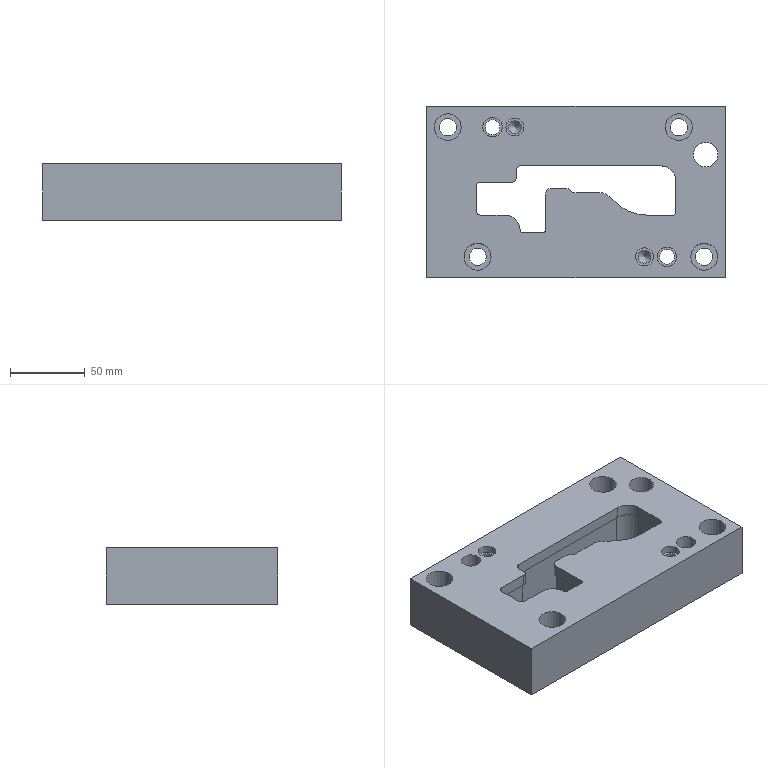Part | STEP file | lll_id214_x_t | 1 solid | 88 faces | box 200 x 115 x 38 mm | volume 675868 mm3 | cylinder 47 | plane 39 | cone 2 | commonest cylinder face diameters 6 x6 9 x4 11.509 x4 18.008 x4 3 x2 4 x2